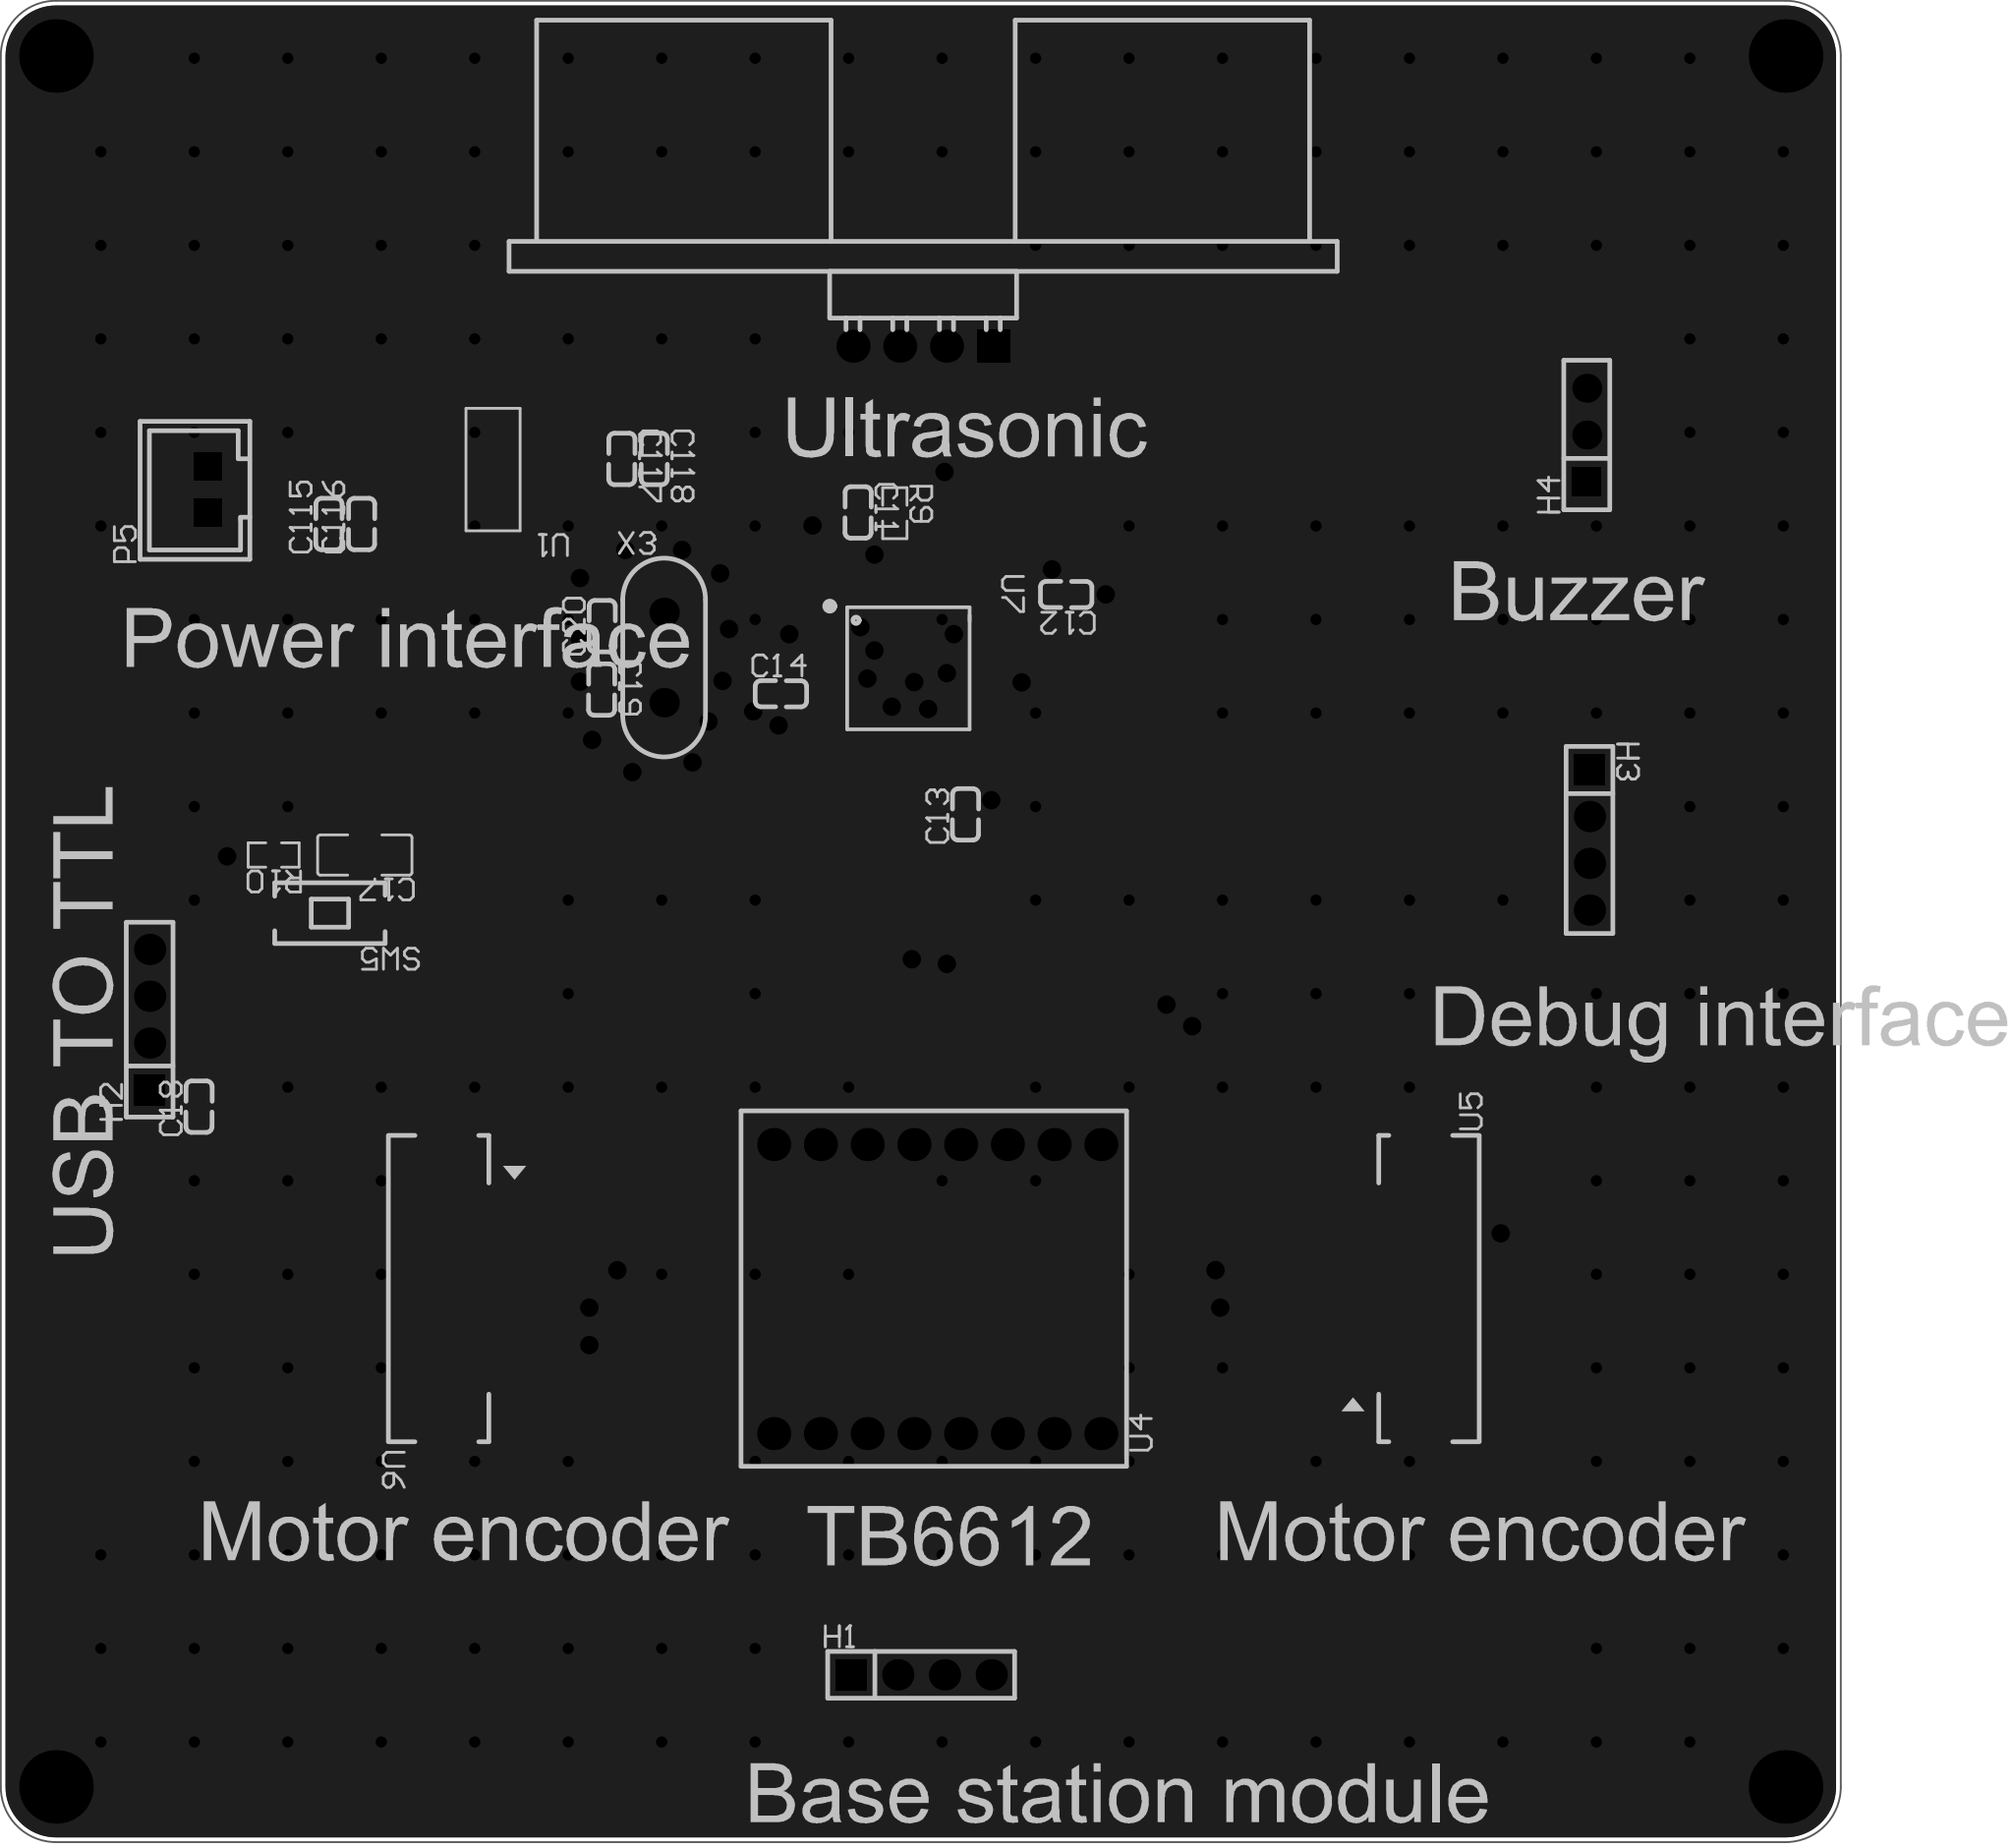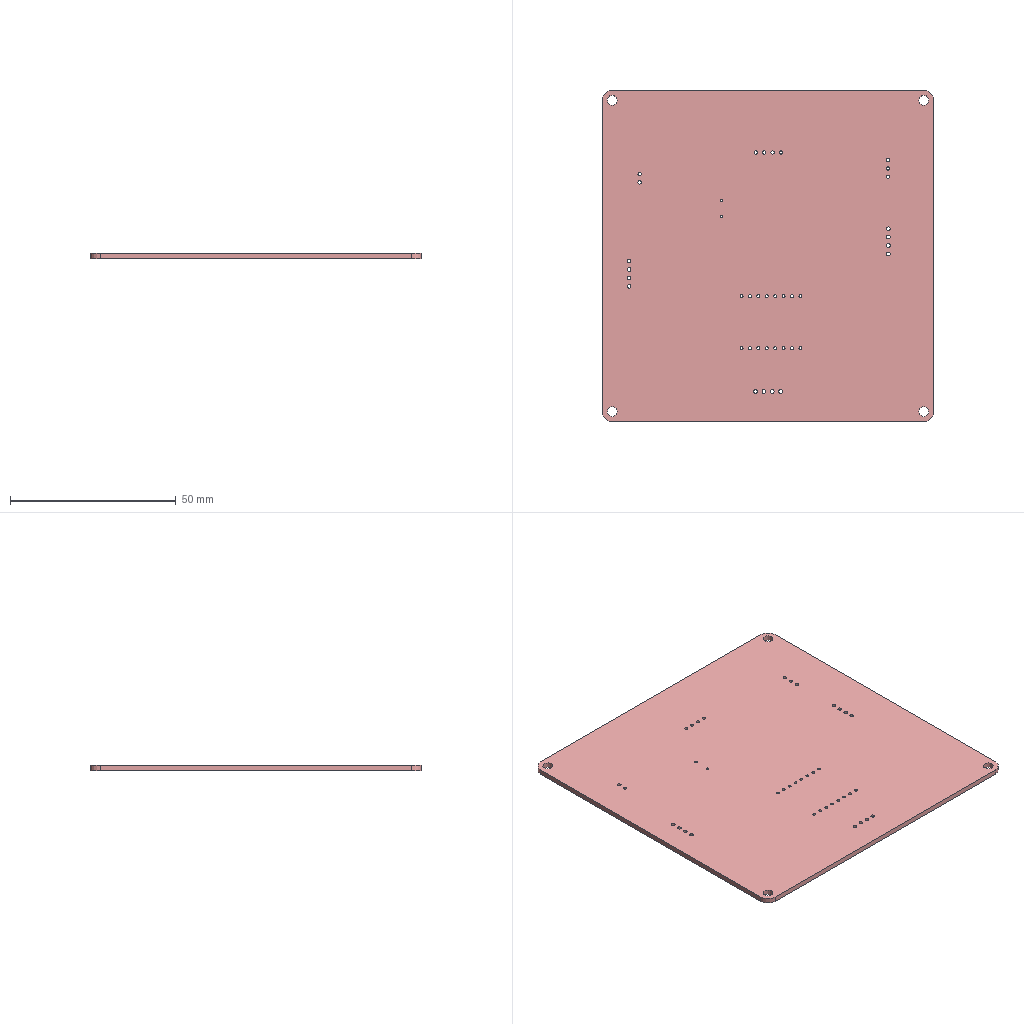Circuit board layout | Altium Designer | box 100 x 100 x 1.6 mm
Layer stack:
# Altium Designer layer stack of  (unit mm; dielectric type: 0 none, 1 core, 2 prepreg, 3 surface material)
index,name,kind,layer,copper_thickness_mm,dielectric_type,dielectric_thickness_mm,dielectric_material,dielectric_constant
0,Top Paste Mask Layer,other,,,,,,
1,Top Silkscreen Layer,other,,,,,,
2,Top Solder Mask Layer,dielectric,,,3,0.01,,3.3
3,Top Layer,copper,Top Layer,0.035,,,,
4,Dielectric1,dielectric,,,3,1.51,FR4,4.5
5,Bottom Layer,copper,Bottom Layer,0.035,,,,
6,Bottom Solder Mask Layer,dielectric,,,3,0.01,,3.3
7,Bottom Silkscreen Layer,other,,,,,,
8,Bottom Paste Mask Layer,other,,,,,,
# drill layer pairs: low layer,high layer
drill_pair,Top Layer,Bottom Layer
Part placement:
Designator,Comment,Layer,Footprint,Center-X(mm),Center-Y(mm),Rotation
U11,HC-SR04,TopLayer,TH_HC-SR04V,141.458,162.072,180
P5,XH2.54 straight socket-2P,TopLayer,CONN-TH_XH2.54-2P,102.583,154.305,90
U5,MXPH-2.0-06P-LT1-0-A,TopLayer,CONN-SMD_6P-P2.00_MXPH-2.0-6P-LT1-0-A,167.363,110.891,270
U6,MXPH-2.0-06P-LT1-0-A,TopLayer,CONN-SMD_6P-P2.00_MXPH-2.0-6P-LT1-0-A,116.713,110.891,90
U4,,TopLayer,tb6612,142.229,110.866,90
H1,,TopLayer,HDR-TH_4P-P2.54-V-M,141.351,89.916,0
H2,,TopLayer,HDR-TH_4P-P2.54-V-F,99.421,125.496,90
H4,,TopLayer,HDR-TH_3P-P2.54-V-F,177.526,157.246,90
C17,100uF,TopLayer,C1206,111.113,134.437,180
C18,100nF,TopLayer,C0603,102.108,120.777,90
C19,20pF,TopLayer,C0603,123.983,143.415,270
C20,20pF,TopLayer,C0603,124.017,146.874,90
C115,10uF,TopLayer,C0603,109.167,152.42,90
C116,100nF,TopLayer,C0603,110.945,152.42,90
C117,100nF,TopLayer,C0603,125.08,155.939,270
C118,10uF,TopLayer,C0603,126.845,155.939,270
R9,10kΩ,TopLayer,R0603,139.92,153.002,270
R10,1kΩ,TopLayer,R0603,106.16,134.437,180
SW5,TS-1101-C-W,TopLayer,SW-SMD_L6.0-W3.3-LS8.0,109.081,131.262,180
U7,STM32F103C8T6,TopLayer,LQFP-48_L7.0-W7.0-P0.50-LS9.0-BL,140.644,144.564,270
X3,8MHz,TopLayer,OSC-TH_L10.0-W4.5-P5.00,127.381,145.161,0
H3,,TopLayer,HDR-TH_4P-P2.54-V-M,177.673,135.255,270
U1,AMS1117-3.3,TopLayer,SOT-223-3_L6.5-W3.4-P2.30-LS7.0-BR,117.983,155.37,180
C11,100nF,TopLayer,C0603,137.922,153.035,270
C12,100nF,TopLayer,C0603,149.225,148.59,180
C13,100nF,TopLayer,C0603,143.764,136.652,90
C14,100nF,TopLayer,C0603,133.737,143.192,0
Pad and via stacks:
# Altium Designer via and pad stacks of  (unit mm). Each distinct definition once, with the count of objects using it.
# via: kind,start_layer,end_layer,hole_mm,diameter_mm,mode(0 simple;1 top-mid-bottom;2 full stack),diameter_per_layer,count,example_net
# pad: kind,layer,hole_mm,hole_type(0 round;1 square;2 slot),plating,top_size,top_shape(1 round;2 rect;3 octagon;9 rounded rect),mid_size,bottom_size,mode,footprint,size_per_layer,count,example
pad,Multi-Layer,3,0,plated,4x4,1,4x4,4x4,0,,,4,1
pad,Multi-Layer,1.001,0,plated,1.8x1.8,1,1.8x1.8,1.8x1.8,0,TH_HC-SR04V,,3,U11.4
pad,Multi-Layer,1.001,0,plated,1.8x1.8,2,1.8x1.8,1.8x1.8,0,TH_HC-SR04V,,1,U11.1
pad,Multi-Layer,1,2,plated,1.524x1.524,2,1.524x1.524,1.524x1.524,0,CONN-TH_XH2.54-2P,,2,P5.1
pad,Multi-Layer,0.9,0,plated,1.8x1.8,1,1.8x1.8,1.8x1.8,0,tb6612,,16,U4.1
pad,Multi-Layer,1.1,0,plated,1.7x1.7,2,1.7x1.7,1.7x1.7,0,HDR-TH_4P-P2.54-V-M,,2,H1.1
pad,Multi-Layer,1.1,0,plated,1.7x1.7,1,1.7x1.7,1.7x1.7,0,HDR-TH_4P-P2.54-V-M,,6,H1.2
pad,Multi-Layer,1.1,0,plated,1.7x1.7,2,1.7x1.7,1.7x1.7,0,HDR-TH_4P-P2.54-V-F,,1,H2.1
pad,Multi-Layer,1.1,0,plated,1.7x1.7,1,1.7x1.7,1.7x1.7,0,HDR-TH_4P-P2.54-V-F,,3,H2.2
pad,Multi-Layer,1.02,0,plated,1.575x1.575,1,1.575x1.575,1.575x1.575,0,HDR-TH_3P-P2.54-V-F,,2,H4.3
pad,Multi-Layer,1.02,0,plated,1.575x1.575,2,1.575x1.575,1.575x1.575,0,HDR-TH_3P-P2.54-V-F,,1,H4.1
pad,Multi-Layer,0.7,0,plated,1.6x1.6,1,1.6x1.6,1.6x1.6,0,OSC-TH_L10.0-W4.5-P5.00,,2,X3.2
pad,Top Layer,0,0,plated,1x5.5,2,1x5.5,1x5.5,0,CONN-SMD_6P-P2.00_MXPH-2.0-6P-LT1-0-A,,12,U5.1
pad,Top Layer,0,0,plated,1.6x3,2,1.6x3,1.6x3,0,CONN-SMD_6P-P2.00_MXPH-2.0-6P-LT1-0-A,,4,U5.8
pad,Top Layer,0,0,plated,1.485x1.728,2,1.485x1.728,1.485x1.728,0,C1206,,2,C17.2
pad,Top Layer,0,0,plated,0.8x0.9,2,0.8x0.9,0.8x0.9,0,C0603,,22,C18.2
pad,Top Layer,0,0,plated,0.8065x0.864,2,0.8065x0.864,0.8065x0.864,0,R0603,,4,R9.2
pad,Top Layer,0,0,plated,1.9x1.5,2,1.9x1.5,1.9x1.5,0,SW-SMD_L6.0-W3.3-LS8.0,,2,SW5.1
pad,Top Layer,0,0,plated,0.27x1.5,1,0.27x1.5,0.27x1.5,0,LQFP-48_L7.0-W7.0-P0.50-LS9.0-BL,,24,U7.1
pad,Top Layer,0,0,plated,1.5x0.27,1,1.5x0.27,1.5x0.27,0,LQFP-48_L7.0-W7.0-P0.50-LS9.0-BL,,24,U7.13
pad,Top Layer,0,0,plated,2.5x1.1,2,2.5x1.1,2.5x1.1,0,SOT-223-3_L6.5-W3.4-P2.30-LS7.0-BR,,3,U1.1
pad,Top Layer,0,0,plated,2.34x3.6,2,2.34x3.6,2.34x3.6,0,SOT-223-3_L6.5-W3.4-P2.30-LS7.0-BR,,1,U1.4
via,Top Layer,Bottom Layer,0.5004,1,0,,41,PA0
via,Top Layer,Bottom Layer,0.3048,0.61,0,,237,GND
Copper pours:
name,layer,net,type(0 solid;1 hatched;2 none)
Bottom Layer-GND,Bottom Layer,GND,0
Top Layer-GND,Top Layer,GND,0
Design rules, without the lines most boards share:
# Altium Designer design rules of  (exported by Altium Designer, unit mm)
# columns: name | kind | enabled | priority | scope1 | scope2 | descriptor | typed fields (field=value)
Copper_copperRegion_copperThickness1oz | 0 | disabled | 4 | All | All | Clearance Constraint (Gap=5.984mil) (Disabled)(All),(All) | gap=0.152
Copper_copperRegion_copperThickness1oz_1 | 63 | disabled | 4 | All | All | Board Clearance Constraint (Gap=0mil) (Disabled)(All) |
Copper_copperRegion_Copper_copperRegion | 0 | disabled | 5 | All | All | Clearance Constraint (Gap=5.984mil) (Disabled)(All),(All) | gap=0.152
Copper_copperRegion_Copper_copperRegion_1 | 63 | disabled | 5 | All | All | Board Clearance Constraint (Gap=0mil) (Disabled)(All) |
copperThickness1oz | 0 | enabled | 6 | All | All | Clearance Constraint (Gap=5.984mil) (All),(All) | gap=0.152
copperThickness1oz_1 | 63 | enabled | 6 | All | All | Board Clearance Constraint (Gap=0mil) (All) |
copperRegion_copperThickness1oz | 20 | disabled | 1 | All | All | Polygon Connect Rule(Relief Connect )(Conductor Width=10mil) (Relief Angle=90 Angle) (Entries=4) (Air Gap Width=10mil) (Disabled)(All),(All) | connect_style(0=relief,1=direct,2=none)=0 relief_conductor_width=0.254 relief_entries=4
copperRegion_Copper_copperRegion | 20 | disabled | 2 | All | All | Polygon Connect Rule(Relief Connect )(Conductor Width=10mil) (Relief Angle=90 Angle) (Entries=4) (Air Gap Width=10mil) (Disabled)(All),(All) | connect_style(0=relief,1=direct,2=none)=0 relief_conductor_width=0.254 relief_entries=4
copperRegion | 20 | enabled | 3 | All | All | Polygon Connect Rule(Relief Connect )(Conductor Width=10mil) (Relief Angle=90 Angle) (Entries=4) (Air Gap Width=10mil) (All),(All) | connect_style(0=relief,1=direct,2=none)=0 relief_conductor_width=0.254 relief_entries=4